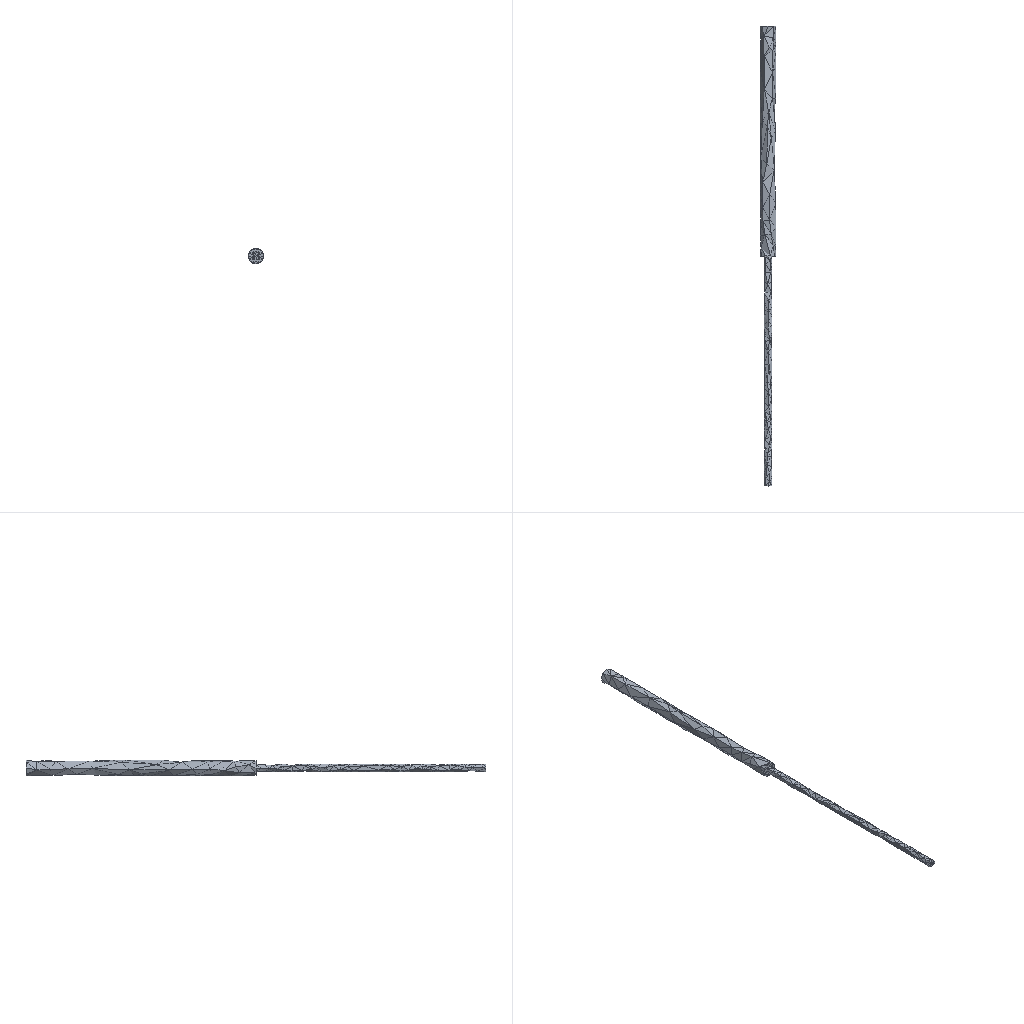Simulation study | ansys workbench
Set-up summary:
category,name,step,type,value,unit,region
solver,ansys_workbench
units,mm-N-s-tonne (MPa),,stated,"/units,MPA"
analysis,LS1,,static
load_step,LS1,LS1,static,nsubst=1; time=1
mesh,nodes,,,1252
mesh,elements,,,582
element_type,SOLID187,,,552
element_type,SURF154,,,30
material,Structural Steel,,E,200000,tonne s^-2 mm^-1
material,Structural Steel,,nu,0.3
material,Structural Steel,,density,7.85e-09,tonne mm^-3
material,Structural Steel,,conductivity,60.5,tonne mm s^-3 C^-1
material,Structural Steel,,specific_heat,4.34e+08,mm^2 s^-2 C^-1
material,Structural Steel,,cte,1.2e-05,C^-1
material,Structural Steel,,permeability,10000
material,Structural Steel,,resistivity,0.00017,ohm mm
load,Define Force Using Surface Effect Elements,LS1,surface-effect pres face 2,-513.134,,SURF154 #2
load,Define Force Using Surface Effect Elements,LS1,surface-effect pres face 2,-192.437,,SURF154 #3
load,Define Force Using Surface Effect Elements,LS1,surface-effect pres face 2,4244.85,,SURF154 #4
bc,Fixed Supports,model,fixed,[dofs=ALL],,_FIXEDSU
bc,Constant Zero Displacement X,model,fixed,[dofs=UX],,_DISPZEROUX
bc,Constant Zero Displacement Z,model,fixed,[dofs=UZ],,_DISPZEROUZ
named_set,_FIXEDSU,,node,42
named_set,_DISPZEROUX,,node,20
named_set,_DISPZEROUZ,,node,20
Ansys APDL input file, long lists of numbers shortened:
/batch
/config,noeldb,1     ! force off writing results to database
*get,_wallstrt,active,,time,wall
! ANSYS input file written by Workbench version 2022 R1
! File used for geometry attach:
/title,1--____ (A5)
! ****** Begin Custom Load Command Snippet ******
/COM, ACT Extensions:
/COM,     LSDYNA, 2021.1
/COM,
! ****** End   Custom Load Command Snippet ******
*DIM,_wb_ProjectScratch_dir,string,248
_wb_ProjectScratch_dir(1) = ''
*DIM,_wb_SolverFiles_dir,string,248
_wb_SolverFiles_dir(1) = ''
*DIM,_wb_userfiles_dir,string,248
_wb_userfiles_dir(1) = ''
/com,--- Data in consistent NMM units. See Solving Units in the help system for more information.
/units,MPA
/nopr
/wb,file,start              !  signify a WB generated input file
/prep7
! Turn off shape checking because checks already performed inside WB mesher.
! See help system for more information.
SHPP,OFF,,NOWARN
/nolist
etcon,set             ! allow ANSYS to choose best KEYOP's for 180x elements, resets any applicable keyopt to MAPDL defaults
/com,*********** Nodes for the whole assembly ***********
nblock,3,,1377
(1i9,3e20.9e3)
        1    -1.000000000E+01     6.000000000E+02    -3.572850612E-16
! (1251 more lines like these left out)
-1
/wb,elem,start            !  set before creation of elements
/com,*********** Elements for Body 1 "SYS\__" ***********
et,1,187
eblock,19,solid,,552
(19i9)
        1        1        1        1        0        0        0        0       10        0        1       86      230       90       95      641      658      637      638
! (1103 more lines like these left out)
-1
/wb,elem,end               !  done creating elements
/com,*********** Send User Defined Coordinate System(s) ***********
csys,0
toffst,273.15,  ! Temperature offset from absolute zero
/com,*********** Set Reference Temperature ***********
tref,22.
/wb,mat,start              !  starting to send materials
/com,*********** Send Materials ***********
Temperature = 'TEMP' ! Temperature
MP,DENS,1,7.85e-09,	! tonne mm^-3
MP,ALPX,1,1.2e-05,	! C^-1
MP,C,1,434000000,	! mm^2 s^-2 C^-1
MP,KXX,1,60.5,	! tonne mm s^-3 C^-1
MP,RSVX,1,0.00017,	! ohm mm
MP,EX,1,200000,	! tonne s^-2 mm^-1
MP,NUXY,1,0.3,
MP,MURX,1,10000,
/wb,mat,end                !  done sending materials
!************************* Model Summary ********************
!SYS\__,	结构钢,	matid,	1
!************************* End Model Summary ********************
! get the diagonal of the bounding box. Needed later for other things
*get,_xmin,node,,mnloc,x
*get,_ymin,node,,mnloc,y
*get,_zmin,node,,mnloc,z
*get,_xmax,node,,mxloc,x
*get,_ymax,node,,mxloc,y
*get,_zmax,node,,mxloc,z
_ASMDIAG=(_xmax-_xmin)*(_xmax-_xmin)+(_ymax-_ymin)*(_ymax-_ymin)+(_zmax-_zmin)*(_zmax-_zmin)
_ASMDIAG=SQRT(_ASMDIAG)
/wb,contact,start          !  starting to send contact
/wb,contact,end            !  done creating contacts
/golist
/wb,load,start             !  starting to send loads
/com,*********** Fixed Supports ***********
CMBLOCK,_FIXEDSU,NODE,       42
(8i10)
         1         2         3         4         5         6         7         8
        27        28        29        30        31        32        33        34
       239       240       243       244       245       250       251       255
       256       257       259       260       264       370       371       376
       377       378       381       382       387       388       389       392
       397       398
cmsel,s,_FIXEDSU
d,all,all
nsel,all
/com,******* Constant Zero Displacement X *******
CMBLOCK,_DISPZEROUX,NODE,       20
(8i10)
         9        10        11        12        13        14        15        16
        17        18       274       275       278       279       283       284
       290       291       297       298
cmsel,s,_DISPZEROUX
d,all,ux,0
nsel,all
/com,******* Constant Zero Displacement Z *******
CMBLOCK,_DISPZEROUZ,NODE,       20
(8i10)
         9        10        11        12        13        14        15        16
        17        18       274       275       278       279       283       284
       290       291       297       298
cmsel,s,_DISPZEROUZ
d,all,uz,0
nsel,all
/com,*********** Define Force Using Surface Effect Elements ***********
local,12,0,0.,0.,0.,0.,0.,0.
csys,0
et,2,154
eblock,10,,,6
(15i9)
     1003        2        2        2       12       31       34       28       28      392      378       28      376
     1004        2        2        2       12       27       34       31       31      371      392       31      370
     1005        2        2        2       12       29       32       33       33      381      397       33      382
     1006        2        2        2       12       34       30       32       32      389      387       32      398
     1007        2        2        2       12       32       30       33       33      387      388       33      397
     1008        2        2        2       12       28       34       32       32      378      398       32      377
-1
esel,s,type,,2
keyop,2,2,1                ! Apply load in local coordinate system
keyop,2,7,1                ! Use original area so load is constant in large deformation
esel,all
/com,*********** Define Force Using Surface Effect Elements ***********
local,13,0,0.,0.,0.,0.,0.,0.
csys,0
et,3,154
eblock,10,,,6
(15i9)
     1009        3        3        3       13        6        2        7        7      244      245        7      264
     1010        3        3        3       13        7        2        5        5      245      243        5      259
     1011        3        3        3       13        7        5        4        4      259      255        4      256
     1012        3        3        3       13        3        6        7        7      250      264        7      251
     1013        3        3        3       13        1        8        5        5      240      260        5      239
     1014        3        3        3       13        4        5        8        8      255      260        8      257
-1
esel,s,type,,3
keyop,3,2,1                ! Apply load in local coordinate system
keyop,3,7,1                ! Use original area so load is constant in large deformation
esel,all
/com,*********** Define Force Using Surface Effect Elements ***********
local,14,0,0.,0.,0.,0.,0.,0.
csys,0
et,4,154
eblock,10,,,18
(15i9)
     1015        4        4        4       14       11       15       25       25      283      307       25      286
! (17 more lines like these left out)
-1
esel,s,type,,4
keyop,4,2,1                ! Apply load in local coordinate system
keyop,4,7,1                ! Use original area so load is constant in large deformation
esel,all
/gst,on,on
fini
*get,_numnode,node,0,count
*get,_numelem,elem,0,count
*get, _MAXELEMNUM, elem, 0, NUM, MAX
*get, _MAXNODENUM, node, 0, NUM, MAX
*get, _MAXELEMTYPE, etyp, 0, NUM, MAX
*get, _MAXREALCONST, real, 0, NUM, MAX
/go
/wb,load,end               !  done creating loads
/com,--- Number of total nodes = %_numnode%
/com,--- Number of contact elements = 30
/com,--- Number of spring elements = 0
/com,--- Number of bearing elements = 0
/com,--- Number of solid elements = 552
/com,--- Number of condensed parts = 0
/com,--- Number of total elements = %_numelem%
*get,_wallbsol,active,,time,wall
/com,****************************************************************************
/com,*************************    SOLUTION       ********************************
/com,****************************************************************************
/solu
antype,0                   ! static analysis
_thickRatio=  0     ! Ratio of thick parts in the model
eqsl,sparse,,,,,1
cntr,print,1               ! print out contact info and also make no initial contact an error
dmpoption,emat,no             ! Don't combine emat file for DANSYS
dmpoption,esav,no             ! Don't combine esav file for DANSYS
nldiag,cont,iter           ! print out contact info each equilibrium iteration
rescontrol,,none                 ! Do not keep any restart files
/com,****************************************************
/com,******************* SOLVE FOR LS 1 OF 1 ****************
esel,s,type,,2
nsle
sfe,all,1,pres,1,0.
sfe,all,2,pres,1,-513.134
sfe,all,3,pres,1,0.
esel,s,type,,3
nsle
sfe,all,1,pres,1,0.
sfe,all,2,pres,1,-192.437
sfe,all,3,pres,1,0.
esel,s,type,,4
nsle
sfe,all,1,pres,1,0.
sfe,all,2,pres,1,4244.847
sfe,all,3,pres,1,0.
nsel,all
esel,all
/nopr
/gopr
nsub,1,1,1
time,1.
outres,erase
outres,all,none
outres,nsol,all,
outres,rsol,all
outres,eangl,all
outres,etmp,all
outres,veng,all
outres,strs,all,
outres,epel,all,
outres,eppl,all,
outres,cont,all,
! *********** WB SOLVE COMMAND ***********
! check interactive state
*get,ANSINTER_,active,,int
*if,ANSINTER_,ne,0,then
/eof
*endif
solve
/com *************** Write FE CONNECTORS *********
CEWRITE,file,ce,,INTE
/com,****************************************************
/com,*************** FINISHED SOLVE FOR LS 1 *************
*get,_wallasol,active,,time,wall
/nopr
*get,_numnode,node,0,count
*get,_numelem,elem,0,count
*get, _MAXELEMNUM, elem, 0, NUM, MAX
*get, _MAXNODENUM, node, 0, NUM, MAX,,,INTERNAL
*get, _MAXELEMTYPE, etyp, 0, NUM, MAX
*get, _MAXREALCONST, real, 0, NUM, MAX
/gopr
/post1
xmlo,ENCODING,ISO-8859-1
xmlo,parm
/xml,parm,xml
fini
/gopr
*get,_walldone,active,,time,wall
_preptime=(_wallbsol-_wallstrt)*3600
_solvtime=(_wallasol-_wallbsol)*3600
_posttime=(_walldone-_wallasol)*3600
_totaltim=(_walldone-_wallstrt)*3600
*get,_dlbratio,active,0,solu,dlbr
*get,_combtime,active,0,solu,comb
*get,_ssmode,active,0,solu,ssmm
*get,_ndofs,active,0,solu,ndof
*get,_sol_end_time,active,0,set,time
*if,_sol_end_time,eq,1.,then
/fclean				!clean distributed files
*endif
/com,--- Total number of nodes = %_numnode%
/com,--- Total number of elements = %_numelem%
/com,--- Element load balance ratio = %_dlbratio%
/com,--- Time to combine distributed files = %_combtime%
/com,--- Sparse memory mode = %_ssmode%
/com,--- Number of DOF = %_ndofs%
/wb,file,end               ! done with WB generated input
Results summary:
result,analyses[0].index,,,1
result,analyses[0].system,,,SYS
result,analyses[0].deck,,,deck.dat
result,analyses[0].solve_status,,,completed
result,analyses[0].analysis_type,,,static
result,analyses[0].physics,,,mechanical
result,analyses[0].unit_system,,,"NMM: mm, ton, N, s, mV, mA, degC"
result,analyses[0].n_sets,,,1
result,analyses[0].load_steps[0].set,set=1,,1
result,analyses[0].load_steps[0].time_or_freq,set=1,,1
result,analyses[0].load_steps[0].max_displacement_magnitude,set=1,,4.016
result,analyses[0].load_steps[0].max_von_mises_nodal,set=1,,4073.45
result,analyses[0].load_steps[0].reaction_force_sum_xyz[1],set=1,,-4.09789e-08
result,analyses[0].load_steps[0].reaction_force_sum_xyz[2],set=1,,-900000
result,analyses[0].load_steps[0].reaction_force_sum_xyz[3],set=1,,3.69425e-09
result,geometry_export[0][0],,,.step
result,geometry_export[0][1],,,ok
result,geometry_export[0][2],,,1